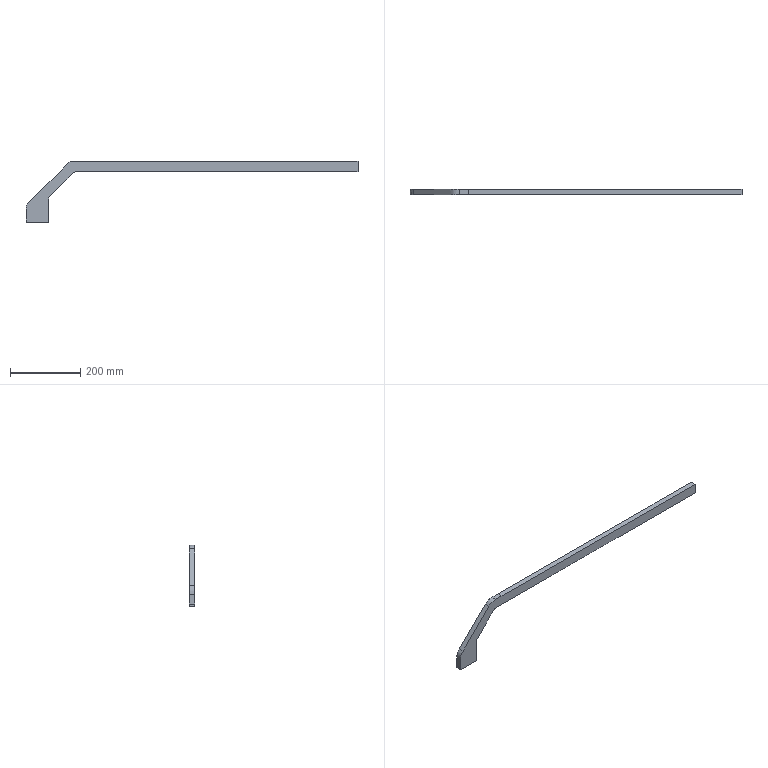Part | NX | features BREP 1 | 1 solid | 18 faces | box 947.785 x 15 x 175.635 mm | volume 489810 mm3 | plane 14 | cylinder 2 | spline 2 | commonest cylinder face diameters 10 x1 20 x1
STEP:
#1=CARTESIAN_POINT('',(752.678,-679.988,1273.821));
#2=VERTEX_POINT('',#1);
#3=CARTESIAN_POINT('',(752.678,-664.988,1273.821));
#4=VERTEX_POINT('',#3);
#5=CARTESIAN_POINT('',(752.678,-672.488,1273.821));
#6=DIRECTION('',(0.,1.,0.));
#7=VECTOR('',#6,1000.);
#8=LINE('',#5,#7);
#9=EDGE_CURVE('',#2,#4,#8,.T.);
#10=ORIENTED_EDGE('',*,*,#9,.T.);
#11=CARTESIAN_POINT('',(754.143,-664.988,1277.356));
#12=VERTEX_POINT('',#11);
#13=CARTESIAN_POINT('',(757.678,-664.988,1273.821));
#14=DIRECTION('',(0.,-1.,0.));
#15=DIRECTION('',(1.,0.,0.));
#16=AXIS2_PLACEMENT_3D('',#13,#14,#15);
#17=CIRCLE('',#16,5.);
#18=EDGE_CURVE('',#12,#4,#17,.T.);
#19=ORIENTED_EDGE('',*,*,#18,.F.);
#20=CARTESIAN_POINT('',(754.143,-679.988,1277.356));
#21=VERTEX_POINT('',#20);
#22=CARTESIAN_POINT('',(754.143,-672.488,1277.356));
#23=DIRECTION('',(0.,1.,0.));
#24=VECTOR('',#23,1000.);
#25=LINE('',#22,#24);
#26=EDGE_CURVE('',#21,#12,#25,.T.);
#27=ORIENTED_EDGE('',*,*,#26,.F.);
#28=CARTESIAN_POINT('',(757.678,-679.988,1273.821));
#29=DIRECTION('',(0.,1.,0.));
#30=DIRECTION('',(1.,0.,0.));
#31=AXIS2_PLACEMENT_3D('',#28,#29,#30);
#32=CIRCLE('',#31,5.);
#33=EDGE_CURVE('',#2,#21,#32,.T.);
#34=ORIENTED_EDGE('',*,*,#33,.F.);
#35=EDGE_LOOP('',(#10,#19,#27,#34));
#36=FACE_BOUND('',#35,.T.);
#37=CARTESIAN_POINT('',(757.678,-672.488,1273.821));
#38=DIRECTION('',(0.,1.,0.));
#39=DIRECTION('',(-1.,0.,0.));
#40=AXIS2_PLACEMENT_3D('',#37,#38,#39);
#41=CYLINDRICAL_SURFACE('',#40,5.);
#42=ADVANCED_FACE('',(#36),#41,.F.);
#43=CARTESIAN_POINT('',(1635.458,-679.988,1378.69));
#44=VERTEX_POINT('',#43);
#45=CARTESIAN_POINT('',(1635.458,-664.988,1378.69));
#46=VERTEX_POINT('',#45);
#47=CARTESIAN_POINT('',(1635.458,-672.488,1378.69));
#48=DIRECTION('',(0.,1.,0.));
#49=VECTOR('',#48,1000.);
#50=LINE('',#47,#49);
#51=EDGE_CURVE('',#44,#46,#50,.T.);
#52=ORIENTED_EDGE('',*,*,#51,.T.);
#53=CARTESIAN_POINT('',(855.477,-664.988,1378.69));
#54=VERTEX_POINT('',#53);
#55=CARTESIAN_POINT('',(1245.467,-664.988,1378.69));
#56=DIRECTION('',(1.,0.,0.));
#57=VECTOR('',#56,1000.);
#58=LINE('',#55,#57);
#59=EDGE_CURVE('',#54,#46,#58,.T.);
#60=ORIENTED_EDGE('',*,*,#59,.F.);
#61=CARTESIAN_POINT('',(855.477,-679.988,1378.69));
#62=VERTEX_POINT('',#61);
#63=CARTESIAN_POINT('',(855.477,-672.488,1378.69));
#64=DIRECTION('',(0.,1.,0.));
#65=VECTOR('',#64,1000.);
#66=LINE('',#63,#65);
#67=EDGE_CURVE('',#62,#54,#66,.T.);
#68=ORIENTED_EDGE('',*,*,#67,.F.);
#69=CARTESIAN_POINT('',(1245.467,-679.988,1378.69));
#70=DIRECTION('',(1.,0.,0.));
#71=VECTOR('',#70,1000.);
#72=LINE('',#69,#71);
#73=EDGE_CURVE('',#62,#44,#72,.T.);
#74=ORIENTED_EDGE('',*,*,#73,.T.);
#75=EDGE_LOOP('',(#52,#60,#68,#74));
#76=FACE_BOUND('',#75,.T.);
#77=CARTESIAN_POINT('',(1245.467,-679.988,1378.69));
#78=DIRECTION('',(0.,0.,1.));
#79=DIRECTION('',(1.,0.,0.));
#80=AXIS2_PLACEMENT_3D('',#77,#78,#79);
#81=PLANE('',#80);
#82=ADVANCED_FACE('',(#76),#81,.T.);
#83=ORIENTED_EDGE('',*,*,#67,.T.);
#84=CARTESIAN_POINT('',(855.475,-664.988,1378.689));
#85=VERTEX_POINT('',#84);
#86=CARTESIAN_POINT('',(855.476,-664.988,1378.689));
#87=DIRECTION('',(0.7071,0.,0.7071));
#88=VECTOR('',#87,1000.);
#89=LINE('',#86,#88);
#90=EDGE_CURVE('',#85,#54,#89,.T.);
#91=ORIENTED_EDGE('',*,*,#90,.F.);
#92=CARTESIAN_POINT('',(855.475,-679.988,1378.689));
#93=VERTEX_POINT('',#92);
#94=CARTESIAN_POINT('',(855.475,-672.488,1378.689));
#95=DIRECTION('',(0.,1.,0.));
#96=VECTOR('',#95,1000.);
#97=LINE('',#94,#96);
#98=EDGE_CURVE('',#93,#85,#97,.T.);
#99=ORIENTED_EDGE('',*,*,#98,.F.);
#100=CARTESIAN_POINT('',(855.476,-679.988,1378.689));
#101=DIRECTION('',(0.7071,0.,0.7071));
#102=VECTOR('',#101,1000.);
#103=LINE('',#100,#102);
#104=EDGE_CURVE('',#93,#62,#103,.T.);
#105=ORIENTED_EDGE('',*,*,#104,.T.);
#106=EDGE_LOOP('',(#83,#91,#99,#105));
#107=FACE_BOUND('',#106,.T.);
#108=CARTESIAN_POINT('',(855.476,-679.988,1378.689));
#109=DIRECTION('',(-0.7071,0.,0.7071));
#110=DIRECTION('',(0.7071,0.,0.7071));
#111=AXIS2_PLACEMENT_3D('',#108,#109,#110);
#112=PLANE('',#111);
#113=ADVANCED_FACE('',(#107),#112,.T.);
#114=ORIENTED_EDGE('',*,*,#98,.T.);
#115=CARTESIAN_POINT('',(829.282,-664.988,1378.689));
#116=VERTEX_POINT('',#115);
#117=CARTESIAN_POINT('',(842.379,-664.988,1378.689));
#118=DIRECTION('',(1.,0.,0.));
#119=VECTOR('',#118,1000.);
#120=LINE('',#117,#119);
#121=EDGE_CURVE('',#116,#85,#120,.T.);
#122=ORIENTED_EDGE('',*,*,#121,.F.);
#123=CARTESIAN_POINT('',(829.282,-679.988,1378.689));
#124=VERTEX_POINT('',#123);
#125=CARTESIAN_POINT('',(829.282,-679.988,1378.689));
#126=DIRECTION('',(0.,1.,0.));
#127=VECTOR('',#126,1000.);
#128=LINE('',#125,#127);
#129=EDGE_CURVE('',#124,#116,#128,.T.);
#130=ORIENTED_EDGE('',*,*,#129,.F.);
#131=CARTESIAN_POINT('',(842.379,-679.988,1378.689));
#132=DIRECTION('',(1.,0.,0.));
#133=VECTOR('',#132,1000.);
#134=LINE('',#131,#133);
#135=EDGE_CURVE('',#124,#93,#134,.T.);
#136=ORIENTED_EDGE('',*,*,#135,.T.);
#137=EDGE_LOOP('',(#114,#122,#130,#136));
#138=FACE_BOUND('',#137,.T.);
#139=CARTESIAN_POINT('',(842.379,-679.988,1378.689));
#140=DIRECTION('',(0.,0.,1.));
#141=DIRECTION('',(1.,0.,0.));
#142=AXIS2_PLACEMENT_3D('',#139,#140,#141);
#143=PLANE('',#142);
#144=ADVANCED_FACE('',(#138),#143,.T.);
#145=ORIENTED_EDGE('',*,*,#129,.T.);
#146=CARTESIAN_POINT('',(802.462,-664.988,1368.101));
#147=VERTEX_POINT('',#146);
#148=CARTESIAN_POINT('',(802.462,-664.988,1368.101));
#149=CARTESIAN_POINT('',(802.713,-664.988,1368.351));
#150=CARTESIAN_POINT('',(803.201,-664.988,1368.831));
#151=CARTESIAN_POINT('',(803.766,-664.988,1369.381));
#152=CARTESIAN_POINT('',(804.526,-664.988,1370.101));
#153=CARTESIAN_POINT('',(805.14,-664.988,1370.666));
#154=CARTESIAN_POINT('',(805.915,-664.988,1371.354));
#155=CARTESIAN_POINT('',(806.881,-664.988,1372.17));
#156=CARTESIAN_POINT('',(808.007,-664.988,1373.064));
#157=CARTESIAN_POINT('',(809.626,-664.988,1374.201));
#158=CARTESIAN_POINT('',(811.67,-664.988,1375.447));
#159=CARTESIAN_POINT('',(813.989,-664.988,1376.546));
#160=CARTESIAN_POINT('',(816.289,-664.988,1377.335));
#161=CARTESIAN_POINT('',(818.163,-664.988,1377.83));
#162=CARTESIAN_POINT('',(819.887,-664.988,1378.167));
#163=CARTESIAN_POINT('',(821.549,-664.988,1378.39));
#164=CARTESIAN_POINT('',(822.722,-664.988,1378.501));
#165=CARTESIAN_POINT('',(823.715,-664.988,1378.574));
#166=CARTESIAN_POINT('',(824.569,-664.988,1378.619));
#167=CARTESIAN_POINT('',(825.586,-664.988,1378.656));
#168=CARTESIAN_POINT('',(826.27,-664.988,1378.67));
#169=CARTESIAN_POINT('',(826.895,-664.988,1378.679));
#170=CARTESIAN_POINT('',(827.459,-664.988,1378.684));
#171=CARTESIAN_POINT('',(827.759,-664.988,1378.686));
#172=CARTESIAN_POINT('',(828.361,-664.988,1378.688));
#173=CARTESIAN_POINT('',(828.884,-664.988,1378.689));
#174=CARTESIAN_POINT('',(829.282,-664.988,1378.689));
#175=B_SPLINE_CURVE_WITH_KNOTS('',3,(#148,#149,#150,#151,#152,#153,#154,#155,#156,#157,#158,#159,#160,#161,#162,#163,#164,#165,#166,#167,#168,#169,#170,#171,#172,#173,#174),.UNSPECIFIED.,.F.,.F.,(4,1,1,1,1,1,1,1,1,1,1,1,1,1,1,1,1,1,1,1,1,1,1,1,4),(0.,0.03125,0.0625,0.09375,0.125,0.1562,0.1875,0.25,0.3125,0.375,0.5,0.5625,0.625,0.6875,0.75,0.7812,0.8125,0.8438,0.875,0.9062,0.9219,0.9375,0.9531,0.9688,1.),.UNSPECIFIED.);
#176=EDGE_CURVE('',#147,#116,#175,.T.);
#177=ORIENTED_EDGE('',*,*,#176,.F.);
#178=CARTESIAN_POINT('',(802.462,-679.988,1368.101));
#179=VERTEX_POINT('',#178);
#180=CARTESIAN_POINT('',(802.462,-672.488,1368.101));
#181=DIRECTION('',(-0.000000001,1.,-0.000000001));
#182=VECTOR('',#181,1000.);
#183=LINE('',#180,#182);
#184=EDGE_CURVE('',#179,#147,#183,.T.);
#185=ORIENTED_EDGE('',*,*,#184,.F.);
#186=CARTESIAN_POINT('',(829.282,-679.988,1378.689));
#187=CARTESIAN_POINT('',(828.885,-679.988,1378.689));
#188=CARTESIAN_POINT('',(828.361,-679.988,1378.688));
#189=CARTESIAN_POINT('',(827.759,-679.988,1378.686));
#190=CARTESIAN_POINT('',(827.458,-679.988,1378.684));
#191=CARTESIAN_POINT('',(826.895,-679.988,1378.679));
#192=CARTESIAN_POINT('',(826.27,-679.988,1378.67));
#193=CARTESIAN_POINT('',(825.586,-679.988,1378.656));
#194=CARTESIAN_POINT('',(824.57,-679.988,1378.619));
#195=CARTESIAN_POINT('',(823.715,-679.988,1378.574));
#196=CARTESIAN_POINT('',(822.723,-679.988,1378.501));
#197=CARTESIAN_POINT('',(821.548,-679.988,1378.39));
#198=CARTESIAN_POINT('',(819.888,-679.988,1378.167));
#199=CARTESIAN_POINT('',(818.163,-679.988,1377.83));
#200=CARTESIAN_POINT('',(816.29,-679.988,1377.335));
#201=CARTESIAN_POINT('',(813.988,-679.988,1376.546));
#202=CARTESIAN_POINT('',(811.67,-679.988,1375.447));
#203=CARTESIAN_POINT('',(809.627,-679.988,1374.202));
#204=CARTESIAN_POINT('',(808.007,-679.988,1373.064));
#205=CARTESIAN_POINT('',(806.882,-679.988,1372.171));
#206=CARTESIAN_POINT('',(805.916,-679.988,1371.355));
#207=CARTESIAN_POINT('',(805.14,-679.988,1370.666));
#208=CARTESIAN_POINT('',(804.527,-679.988,1370.102));
#209=CARTESIAN_POINT('',(803.766,-679.988,1369.381));
#210=CARTESIAN_POINT('',(803.201,-679.988,1368.832));
#211=CARTESIAN_POINT('',(802.713,-679.988,1368.351));
#212=CARTESIAN_POINT('',(802.462,-679.988,1368.101));
#213=B_SPLINE_CURVE_WITH_KNOTS('',3,(#186,#187,#188,#189,#190,#191,#192,#193,#194,#195,#196,#197,#198,#199,#200,#201,#202,#203,#204,#205,#206,#207,#208,#209,#210,#211,#212),.UNSPECIFIED.,.F.,.F.,(4,1,1,1,1,1,1,1,1,1,1,1,1,1,1,1,1,1,1,1,1,1,1,1,4),(0.,0.03125,0.04688,0.0625,0.07812,0.09375,0.125,0.1562,0.1875,0.2188,0.25,0.3125,0.375,0.4375,0.5,0.625,0.6875,0.75,0.8125,0.8438,0.875,0.9062,0.9375,0.9688,1.),.UNSPECIFIED.);
#214=EDGE_CURVE('',#179,#124,#213,.F.);
#215=ORIENTED_EDGE('',*,*,#214,.T.);
#216=EDGE_LOOP('',(#145,#177,#185,#215));
#217=FACE_BOUND('',#216,.T.);
#218=CARTESIAN_POINT('',(802.462,-680.078,1368.101));
#219=CARTESIAN_POINT('',(802.462,-664.988,1368.101));
#220=CARTESIAN_POINT('',(804.233,-680.078,1369.859));
#221=CARTESIAN_POINT('',(804.233,-664.988,1369.859));
#222=CARTESIAN_POINT('',(807.883,-680.078,1373.32));
#223=CARTESIAN_POINT('',(807.883,-664.988,1373.32));
#224=CARTESIAN_POINT('',(814.437,-680.078,1377.09));
#225=CARTESIAN_POINT('',(814.437,-664.988,1377.09));
#226=CARTESIAN_POINT('',(821.879,-680.078,1378.678));
#227=CARTESIAN_POINT('',(821.879,-664.988,1378.678));
#228=CARTESIAN_POINT('',(826.788,-680.078,1378.689));
#229=CARTESIAN_POINT('',(826.788,-664.988,1378.689));
#230=CARTESIAN_POINT('',(829.282,-680.078,1378.689));
#231=CARTESIAN_POINT('',(829.282,-664.988,1378.689));
#232=B_SPLINE_SURFACE_WITH_KNOTS('',3,1,((#218,#219),(#220,#221),(#222,#223),(#224,#225),(#226,#227),(#228,#229),(#230,#231)),.SURF_OF_LINEAR_EXTRUSION.,.F.,.F.,.F.,(4,1,1,1,4),(2,2),(0.009839,7.507,15.005,22.502,30.),(0.,1.),.UNSPECIFIED.);
#233=ADVANCED_FACE('',(#217),#232,.T.);
#234=ORIENTED_EDGE('',*,*,#184,.T.);
#235=CARTESIAN_POINT('',(698.27,-664.988,1263.91));
#236=VERTEX_POINT('',#235);
#237=CARTESIAN_POINT('',(750.366,-664.988,1316.006));
#238=DIRECTION('',(0.7071,0.,0.7071));
#239=VECTOR('',#238,1000.);
#240=LINE('',#237,#239);
#241=EDGE_CURVE('',#236,#147,#240,.T.);
#242=ORIENTED_EDGE('',*,*,#241,.F.);
#243=CARTESIAN_POINT('',(698.27,-679.988,1263.91));
#244=VERTEX_POINT('',#243);
#245=CARTESIAN_POINT('',(698.27,-679.988,1263.91));
#246=DIRECTION('',(0.,1.,0.));
#247=VECTOR('',#246,1000.);
#248=LINE('',#245,#247);
#249=EDGE_CURVE('',#244,#236,#248,.T.);
#250=ORIENTED_EDGE('',*,*,#249,.F.);
#251=CARTESIAN_POINT('',(750.366,-679.988,1316.006));
#252=DIRECTION('',(0.7071,0.,0.7071));
#253=VECTOR('',#252,1000.);
#254=LINE('',#251,#253);
#255=EDGE_CURVE('',#244,#179,#254,.T.);
#256=ORIENTED_EDGE('',*,*,#255,.T.);
#257=EDGE_LOOP('',(#234,#242,#250,#256));
#258=FACE_BOUND('',#257,.T.);
#259=CARTESIAN_POINT('',(750.366,-679.988,1316.006));
#260=DIRECTION('',(0.7071,0.,-0.7071));
#261=DIRECTION('',(0.7071,0.,0.7071));
#262=AXIS2_PLACEMENT_3D('',#259,#260,#261);
#263=PLANE('',#262);
#264=ADVANCED_FACE('',(#258),#263,.F.);
#265=ORIENTED_EDGE('',*,*,#249,.T.);
#266=CARTESIAN_POINT('',(687.713,-664.988,1240.892));
#267=VERTEX_POINT('',#266);
#268=CARTESIAN_POINT('',(687.713,-664.988,1240.892));
#269=CARTESIAN_POINT('',(687.73,-664.988,1241.481));
#270=CARTESIAN_POINT('',(687.784,-664.988,1242.634));
#271=CARTESIAN_POINT('',(687.896,-664.988,1244.111));
#272=CARTESIAN_POINT('',(688.103,-664.988,1245.85));
#273=CARTESIAN_POINT('',(688.36,-664.988,1247.36));
#274=CARTESIAN_POINT('',(688.735,-664.988,1249.013));
#275=CARTESIAN_POINT('',(689.327,-664.988,1251.048));
#276=CARTESIAN_POINT('',(690.152,-664.988,1253.12));
#277=CARTESIAN_POINT('',(691.126,-664.988,1255.013));
#278=CARTESIAN_POINT('',(691.989,-664.988,1256.459));
#279=CARTESIAN_POINT('',(692.852,-664.988,1257.738));
#280=CARTESIAN_POINT('',(693.907,-664.988,1259.135));
#281=CARTESIAN_POINT('',(694.838,-664.988,1260.259));
#282=CARTESIAN_POINT('',(695.851,-664.988,1261.396));
#283=CARTESIAN_POINT('',(696.523,-664.988,1262.114));
#284=CARTESIAN_POINT('',(697.15,-664.988,1262.77));
#285=CARTESIAN_POINT('',(697.637,-664.988,1263.269));
#286=CARTESIAN_POINT('',(698.054,-664.988,1263.692));
#287=CARTESIAN_POINT('',(698.27,-664.988,1263.91));
#288=B_SPLINE_CURVE_WITH_KNOTS('',3,(#268,#269,#270,#271,#272,#273,#274,#275,#276,#277,#278,#279,#280,#281,#282,#283,#284,#285,#286,#287),.UNSPECIFIED.,.F.,.F.,(4,1,1,1,1,1,1,1,1,1,1,1,1,1,1,1,1,4),(0.,0.0625,0.125,0.1875,0.25,0.3125,0.375,0.5,0.5625,0.625,0.6875,0.75,0.8125,0.875,0.9062,0.9375,0.9688,1.),.UNSPECIFIED.);
#289=EDGE_CURVE('',#267,#236,#288,.T.);
#290=ORIENTED_EDGE('',*,*,#289,.F.);
#291=CARTESIAN_POINT('',(687.674,-664.988,1237.08));
#292=VERTEX_POINT('',#291);
#293=CARTESIAN_POINT('',(687.674,-664.988,1237.08));
#294=CARTESIAN_POINT('',(687.674,-664.988,1237.501));
#295=CARTESIAN_POINT('',(687.674,-664.988,1238.045));
#296=CARTESIAN_POINT('',(687.677,-664.988,1238.654));
#297=CARTESIAN_POINT('',(687.678,-664.988,1238.934));
#298=CARTESIAN_POINT('',(687.684,-664.988,1239.516));
#299=CARTESIAN_POINT('',(687.693,-664.988,1240.145));
#300=CARTESIAN_POINT('',(687.704,-664.988,1240.607));
#301=CARTESIAN_POINT('',(687.713,-664.988,1240.892));
#302=B_SPLINE_CURVE_WITH_KNOTS('',3,(#293,#294,#295,#296,#297,#298,#299,#300,#301),.UNSPECIFIED.,.F.,.F.,(4,1,1,1,1,1,4),(0.,0.25,0.375,0.5,0.625,0.75,1.),.UNSPECIFIED.);
#303=EDGE_CURVE('',#292,#267,#302,.T.);
#304=ORIENTED_EDGE('',*,*,#303,.F.);
#305=CARTESIAN_POINT('',(687.674,-679.988,1237.08));
#306=VERTEX_POINT('',#305);
#307=CARTESIAN_POINT('',(687.674,-672.488,1237.08));
#308=DIRECTION('',(0.,1.,0.));
#309=VECTOR('',#308,1000.);
#310=LINE('',#307,#309);
#311=EDGE_CURVE('',#306,#292,#310,.T.);
#312=ORIENTED_EDGE('',*,*,#311,.F.);
#313=CARTESIAN_POINT('',(687.713,-679.988,1240.892));
#314=VERTEX_POINT('',#313);
#315=CARTESIAN_POINT('',(687.713,-679.988,1240.892));
#316=CARTESIAN_POINT('',(687.704,-679.988,1240.607));
#317=CARTESIAN_POINT('',(687.693,-679.988,1240.146));
#318=CARTESIAN_POINT('',(687.684,-679.988,1239.516));
#319=CARTESIAN_POINT('',(687.678,-679.988,1238.933));
#320=CARTESIAN_POINT('',(687.677,-679.988,1238.655));
#321=CARTESIAN_POINT('',(687.674,-679.988,1238.045));
#322=CARTESIAN_POINT('',(687.674,-679.988,1237.501));
#323=CARTESIAN_POINT('',(687.674,-679.988,1237.08));
#324=B_SPLINE_CURVE_WITH_KNOTS('',3,(#315,#316,#317,#318,#319,#320,#321,#322,#323),.UNSPECIFIED.,.F.,.F.,(4,1,1,1,1,1,4),(0.,0.25,0.375,0.5,0.625,0.75,1.),.UNSPECIFIED.);
#325=EDGE_CURVE('',#306,#314,#324,.F.);
#326=ORIENTED_EDGE('',*,*,#325,.T.);
#327=CARTESIAN_POINT('',(698.27,-679.988,1263.91));
#328=CARTESIAN_POINT('',(698.054,-679.988,1263.692));
#329=CARTESIAN_POINT('',(697.637,-679.988,1263.27));
#330=CARTESIAN_POINT('',(697.149,-679.988,1262.77));
#331=CARTESIAN_POINT('',(696.524,-679.988,1262.115));
#332=CARTESIAN_POINT('',(695.851,-679.988,1261.395));
#333=CARTESIAN_POINT('',(694.839,-679.988,1260.26));
#334=CARTESIAN_POINT('',(693.907,-679.988,1259.134));
#335=CARTESIAN_POINT('',(692.853,-679.988,1257.739));
#336=CARTESIAN_POINT('',(691.989,-679.988,1256.459));
#337=CARTESIAN_POINT('',(691.126,-679.988,1255.013));
#338=CARTESIAN_POINT('',(690.152,-679.988,1253.12));
#339=CARTESIAN_POINT('',(689.327,-679.988,1251.048));
#340=CARTESIAN_POINT('',(688.735,-679.988,1249.014));
#341=CARTESIAN_POINT('',(688.36,-679.988,1247.359));
#342=CARTESIAN_POINT('',(688.104,-679.988,1245.851));
#343=CARTESIAN_POINT('',(687.896,-679.988,1244.111));
#344=CARTESIAN_POINT('',(687.784,-679.988,1242.634));
#345=CARTESIAN_POINT('',(687.73,-679.988,1241.481));
#346=CARTESIAN_POINT('',(687.713,-679.988,1240.892));
#347=B_SPLINE_CURVE_WITH_KNOTS('',3,(#327,#328,#329,#330,#331,#332,#333,#334,#335,#336,#337,#338,#339,#340,#341,#342,#343,#344,#345,#346),.UNSPECIFIED.,.F.,.F.,(4,1,1,1,1,1,1,1,1,1,1,1,1,1,1,1,1,4),(0.,0.03125,0.0625,0.09375,0.125,0.1875,0.25,0.3125,0.375,0.4375,0.5,0.625,0.6875,0.75,0.8125,0.875,0.9375,1.),.UNSPECIFIED.);
#348=EDGE_CURVE('',#314,#244,#347,.F.);
#349=ORIENTED_EDGE('',*,*,#348,.T.);
#350=EDGE_LOOP('',(#265,#290,#304,#312,#326,#349));
#351=FACE_BOUND('',#350,.T.);
#352=CARTESIAN_POINT('',(687.674,-679.988,1237.08));
#353=CARTESIAN_POINT('',(687.674,-664.988,1237.08));
#354=CARTESIAN_POINT('',(687.674,-679.988,1239.588));
#355=CARTESIAN_POINT('',(687.674,-664.988,1239.588));
#356=CARTESIAN_POINT('',(687.693,-679.988,1244.589));
#357=CARTESIAN_POINT('',(687.693,-664.988,1244.589));
#358=CARTESIAN_POINT('',(689.287,-679.988,1251.958));
#359=CARTESIAN_POINT('',(689.287,-664.988,1251.958));
#360=CARTESIAN_POINT('',(693.086,-679.988,1258.533));
#361=CARTESIAN_POINT('',(693.086,-664.988,1258.533));
#362=CARTESIAN_POINT('',(696.506,-679.988,1262.133));
#363=CARTESIAN_POINT('',(696.506,-664.988,1262.133));
#364=CARTESIAN_POINT('',(698.27,-679.988,1263.91));
#365=CARTESIAN_POINT('',(698.27,-664.988,1263.91));
#366=B_SPLINE_SURFACE_WITH_KNOTS('',3,1,((#352,#353),(#354,#355),(#356,#357),(#358,#359),(#360,#361),(#362,#363),(#364,#365)),.SURF_OF_LINEAR_EXTRUSION.,.F.,.F.,.F.,(4,1,1,1,4),(2,2),(0.,7.493,14.985,22.478,29.971),(0.,1.),.UNSPECIFIED.);
#367=ADVANCED_FACE('',(#351),#366,.T.);
#368=ORIENTED_EDGE('',*,*,#311,.T.);
#369=CARTESIAN_POINT('',(687.674,-664.988,1210.887));
#370=VERTEX_POINT('',#369);
#371=CARTESIAN_POINT('',(687.674,-664.988,1223.984));
#372=DIRECTION('',(0.,0.,1.));
#373=VECTOR('',#372,1000.);
#374=LINE('',#371,#373);
#375=EDGE_CURVE('',#370,#292,#374,.T.);
#376=ORIENTED_EDGE('',*,*,#375,.F.);
#377=CARTESIAN_POINT('',(687.674,-679.988,1210.887));
#378=VERTEX_POINT('',#377);
#379=CARTESIAN_POINT('',(687.674,-672.488,1210.887));
#380=DIRECTION('',(0.,-1.,0.));
#381=VECTOR('',#380,1000.);
#382=LINE('',#379,#381);
#383=EDGE_CURVE('',#370,#378,#382,.T.);
#384=ORIENTED_EDGE('',*,*,#383,.T.);
#385=CARTESIAN_POINT('',(687.674,-679.988,1223.984));
#386=DIRECTION('',(0.,0.,1.));
#387=VECTOR('',#386,1000.);
#388=LINE('',#385,#387);
#389=EDGE_CURVE('',#378,#306,#388,.T.);
#390=ORIENTED_EDGE('',*,*,#389,.T.);
#391=EDGE_LOOP('',(#368,#376,#384,#390));
#392=FACE_BOUND('',#391,.T.);
#393=CARTESIAN_POINT('',(687.674,-679.988,1223.984));
#394=DIRECTION('',(1.,0.,0.));
#395=DIRECTION('',(0.,1.,0.));
#396=AXIS2_PLACEMENT_3D('',#393,#394,#395);
#397=PLANE('',#396);
#398=ADVANCED_FACE('',(#392),#397,.F.);
#399=CARTESIAN_POINT('',(687.678,-679.988,1210.892));
#400=VERTEX_POINT('',#399);
#401=CARTESIAN_POINT('',(687.676,-679.988,1210.889));
#402=DIRECTION('',(0.7071,0.,0.7071));
#403=VECTOR('',#402,1000.);
#404=LINE('',#401,#403);
#405=EDGE_CURVE('',#378,#400,#404,.T.);
#406=ORIENTED_EDGE('',*,*,#405,.F.);
#407=ORIENTED_EDGE('',*,*,#383,.F.);
#408=CARTESIAN_POINT('',(687.678,-664.988,1210.892));
#409=VERTEX_POINT('',#408);
#410=CARTESIAN_POINT('',(687.676,-664.988,1210.889));
#411=DIRECTION('',(0.7071,0.,0.7071));
#412=VECTOR('',#411,1000.);
#413=LINE('',#410,#412);
#414=EDGE_CURVE('',#370,#409,#413,.T.);
#415=ORIENTED_EDGE('',*,*,#414,.T.);
#416=CARTESIAN_POINT('',(687.678,-672.488,1210.892));
#417=DIRECTION('',(0.,-1.,0.));
#418=VECTOR('',#417,1000.);
#419=LINE('',#416,#418);
#420=EDGE_CURVE('',#409,#400,#419,.T.);
#421=ORIENTED_EDGE('',*,*,#420,.T.);
#422=EDGE_LOOP('',(#406,#407,#415,#421));
#423=FACE_BOUND('',#422,.T.);
#424=CARTESIAN_POINT('',(687.676,-679.988,1210.889));
#425=DIRECTION('',(0.7071,0.,-0.7071));
#426=DIRECTION('',(0.7071,0.,0.7071));
#427=AXIS2_PLACEMENT_3D('',#424,#425,#426);
#428=PLANE('',#427);
#429=ADVANCED_FACE('',(#423),#428,.T.);
#430=CARTESIAN_POINT('',(687.678,-679.988,1203.055));
#431=VERTEX_POINT('',#430);
#432=CARTESIAN_POINT('',(687.678,-679.988,1206.973));
#433=DIRECTION('',(0.,0.,1.));
#434=VECTOR('',#433,1000.);
#435=LINE('',#432,#434);
#436=EDGE_CURVE('',#431,#400,#435,.T.);
#437=ORIENTED_EDGE('',*,*,#436,.T.);
#438=ORIENTED_EDGE('',*,*,#420,.F.);
#439=CARTESIAN_POINT('',(687.678,-664.988,1203.055));
#440=VERTEX_POINT('',#439);
#441=CARTESIAN_POINT('',(687.678,-664.988,1206.973));
#442=DIRECTION('',(0.,0.,1.));
#443=VECTOR('',#442,1000.);
#444=LINE('',#441,#443);
#445=EDGE_CURVE('',#440,#409,#444,.T.);
#446=ORIENTED_EDGE('',*,*,#445,.F.);
#447=CARTESIAN_POINT('',(687.678,-672.488,1203.055));
#448=DIRECTION('',(0.,1.,0.));
#449=VECTOR('',#448,1000.);
#450=LINE('',#447,#449);
#451=EDGE_CURVE('',#431,#440,#450,.T.);
#452=ORIENTED_EDGE('',*,*,#451,.F.);
#453=EDGE_LOOP('',(#437,#438,#446,#452));
#454=FACE_BOUND('',#453,.T.);
#455=CARTESIAN_POINT('',(687.678,-679.988,655.446));
#456=DIRECTION('',(-1.,0.,0.));
#457=DIRECTION('',(0.,1.,0.));
#458=AXIS2_PLACEMENT_3D('',#455,#456,#457);
#459=PLANE('',#458);
#460=ADVANCED_FACE('',(#454),#459,.T.);
#461=ORIENTED_EDGE('',*,*,#451,.T.);
#462=CARTESIAN_POINT('',(752.678,-664.988,1203.055));
#463=VERTEX_POINT('',#462);
#464=CARTESIAN_POINT('',(720.178,-664.988,1203.055));
#465=DIRECTION('',(1.,0.,0.));
#466=VECTOR('',#465,1000.);
#467=LINE('',#464,#466);
#468=EDGE_CURVE('',#440,#463,#467,.T.);
#469=ORIENTED_EDGE('',*,*,#468,.T.);
#470=CARTESIAN_POINT('',(752.678,-679.988,1203.055));
#471=VERTEX_POINT('',#470);
#472=CARTESIAN_POINT('',(752.678,-672.488,1203.055));
#473=DIRECTION('',(0.,1.,0.));
#474=VECTOR('',#473,1000.);
#475=LINE('',#472,#474);
#476=EDGE_CURVE('',#471,#463,#475,.T.);
#477=ORIENTED_EDGE('',*,*,#476,.F.);
#478=CARTESIAN_POINT('',(720.178,-679.988,1203.055));
#479=DIRECTION('',(1.,0.,0.));
#480=VECTOR('',#479,1000.);
#481=LINE('',#478,#480);
#482=EDGE_CURVE('',#431,#471,#481,.T.);
#483=ORIENTED_EDGE('',*,*,#482,.F.);
#484=EDGE_LOOP('',(#461,#469,#477,#483));
#485=FACE_BOUND('',#484,.T.);
#486=CARTESIAN_POINT('',(717.678,-679.988,1203.055));
#487=DIRECTION('',(0.,0.,-1.));
#488=DIRECTION('',(1.,0.,0.));
#489=AXIS2_PLACEMENT_3D('',#486,#487,#488);
#490=PLANE('',#489);
#491=ADVANCED_FACE('',(#485),#490,.T.);
#492=ORIENTED_EDGE('',*,*,#9,.F.);
#493=CARTESIAN_POINT('',(752.678,-679.988,1238.438));
#494=DIRECTION('',(0.,0.,-1.));
#495=VECTOR('',#494,1000.);
#496=LINE('',#493,#495);
#497=EDGE_CURVE('',#2,#471,#496,.T.);
#498=ORIENTED_EDGE('',*,*,#497,.T.);
#499=ORIENTED_EDGE('',*,*,#476,.T.);
#500=CARTESIAN_POINT('',(752.678,-664.988,1238.438));
#501=DIRECTION('',(0.,0.,-1.));
#502=VECTOR('',#501,1000.);
#503=LINE('',#500,#502);
#504=EDGE_CURVE('',#4,#463,#503,.T.);
#505=ORIENTED_EDGE('',*,*,#504,.F.);
#506=EDGE_LOOP('',(#492,#498,#499,#505));
#507=FACE_BOUND('',#506,.T.);
#508=CARTESIAN_POINT('',(752.678,-672.488,1203.055));
#509=DIRECTION('',(-1.,0.,0.));
#510=DIRECTION('',(0.,1.,0.));
#511=AXIS2_PLACEMENT_3D('',#508,#509,#510);
#512=PLANE('',#511);
#513=ADVANCED_FACE('',(#507),#512,.F.);
#514=CARTESIAN_POINT('',(822.548,-664.988,1345.761));
#515=VERTEX_POINT('',#514);
#516=CARTESIAN_POINT('',(788.345,-664.988,1311.559));
#517=DIRECTION('',(0.7071,0.,0.7071));
#518=VECTOR('',#517,1000.);
#519=LINE('',#516,#518);
#520=EDGE_CURVE('',#12,#515,#519,.T.);
#521=ORIENTED_EDGE('',*,*,#520,.T.);
#522=CARTESIAN_POINT('',(822.548,-679.988,1345.761));
#523=VERTEX_POINT('',#522);
#524=CARTESIAN_POINT('',(822.548,-672.488,1345.761));
#525=DIRECTION('',(0.,-1.,0.));
#526=VECTOR('',#525,1000.);
#527=LINE('',#524,#526);
#528=EDGE_CURVE('',#515,#523,#527,.T.);
#529=ORIENTED_EDGE('',*,*,#528,.T.);
#530=CARTESIAN_POINT('',(788.345,-679.988,1311.559));
#531=DIRECTION('',(0.7071,0.,0.7071));
#532=VECTOR('',#531,1000.);
#533=LINE('',#530,#532);
#534=EDGE_CURVE('',#21,#523,#533,.T.);
#535=ORIENTED_EDGE('',*,*,#534,.F.);
#536=ORIENTED_EDGE('',*,*,#26,.T.);
#537=EDGE_LOOP('',(#521,#529,#535,#536));
#538=FACE_BOUND('',#537,.T.);
#539=CARTESIAN_POINT('',(771.577,-679.988,1294.791));
#540=DIRECTION('',(0.7071,0.,-0.7071));
#541=DIRECTION('',(0.7071,0.,0.7071));
#542=AXIS2_PLACEMENT_3D('',#539,#540,#541);
#543=PLANE('',#542);
#544=ADVANCED_FACE('',(#538),#543,.T.);
#545=ORIENTED_EDGE('',*,*,#534,.T.);
#546=CARTESIAN_POINT('',(829.619,-679.988,1348.69));
#547=VERTEX_POINT('',#546);
#548=CARTESIAN_POINT('',(829.619,-679.988,1338.69));
#549=DIRECTION('',(0.,-1.,0.));
#550=DIRECTION('',(1.,0.,0.));
#551=AXIS2_PLACEMENT_3D('',#548,#549,#550);
#552=CIRCLE('',#551,10.);
#553=EDGE_CURVE('',#547,#523,#552,.T.);
#554=ORIENTED_EDGE('',*,*,#553,.F.);
#555=CARTESIAN_POINT('',(1635.458,-679.988,1348.69));
#556=VERTEX_POINT('',#555);
#557=CARTESIAN_POINT('',(1232.539,-679.988,1348.69));
#558=DIRECTION('',(1.,0.,0.));
#559=VECTOR('',#558,1000.);
#560=LINE('',#557,#559);
#561=EDGE_CURVE('',#547,#556,#560,.T.);
#562=ORIENTED_EDGE('',*,*,#561,.T.);
#563=CARTESIAN_POINT('',(1635.458,-679.988,1363.69));
#564=DIRECTION('',(0.,0.,-1.));
#565=VECTOR('',#564,1000.);
#566=LINE('',#563,#565);
#567=EDGE_CURVE('',#44,#556,#566,.T.);
#568=ORIENTED_EDGE('',*,*,#567,.F.);
#569=ORIENTED_EDGE('',*,*,#73,.F.);
#570=ORIENTED_EDGE('',*,*,#104,.F.);
#571=ORIENTED_EDGE('',*,*,#135,.F.);
#572=ORIENTED_EDGE('',*,*,#214,.F.);
#573=ORIENTED_EDGE('',*,*,#255,.F.);
#574=ORIENTED_EDGE('',*,*,#348,.F.);
#575=ORIENTED_EDGE('',*,*,#325,.F.);
#576=ORIENTED_EDGE('',*,*,#389,.F.);
#577=ORIENTED_EDGE('',*,*,#405,.T.);
#578=ORIENTED_EDGE('',*,*,#436,.F.);
#579=ORIENTED_EDGE('',*,*,#482,.T.);
#580=ORIENTED_EDGE('',*,*,#497,.F.);
#581=ORIENTED_EDGE('',*,*,#33,.T.);
#582=EDGE_LOOP('',(#545,#554,#562,#568,#569,#570,#571,#572,#573,#574,#575,#576,#577,#578,#579,#580,#581));
#583=FACE_BOUND('',#582,.T.);
#584=CARTESIAN_POINT('',(1125.65,-679.988,1648.863));
#585=DIRECTION('',(0.,1.,0.));
#586=DIRECTION('',(-0.7071,0.,0.7071));
#587=AXIS2_PLACEMENT_3D('',#584,#585,#586);
#588=PLANE('',#587);
#589=ADVANCED_FACE('',(#583),#588,.F.);
#590=CARTESIAN_POINT('',(1635.458,-664.988,1348.69));
#591=VERTEX_POINT('',#590);
#592=CARTESIAN_POINT('',(1635.458,-672.488,1348.69));
#593=DIRECTION('',(0.,1.,0.));
#594=VECTOR('',#593,1000.);
#595=LINE('',#592,#594);
#596=EDGE_CURVE('',#556,#591,#595,.T.);
#597=ORIENTED_EDGE('',*,*,#596,.T.);
#598=CARTESIAN_POINT('',(1635.458,-664.988,1363.69));
#599=DIRECTION('',(0.,0.,-1.));
#600=VECTOR('',#599,1000.);
#601=LINE('',#598,#600);
#602=EDGE_CURVE('',#46,#591,#601,.T.);
#603=ORIENTED_EDGE('',*,*,#602,.F.);
#604=ORIENTED_EDGE('',*,*,#51,.F.);
#605=ORIENTED_EDGE('',*,*,#567,.T.);
#606=EDGE_LOOP('',(#597,#603,#604,#605));
#607=FACE_BOUND('',#606,.T.);
#608=CARTESIAN_POINT('',(1635.458,-679.988,1363.69));
#609=DIRECTION('',(-1.,0.,0.));
#610=DIRECTION('',(0.,1.,0.));
#611=AXIS2_PLACEMENT_3D('',#608,#609,#610);
#612=PLANE('',#611);
#613=ADVANCED_FACE('',(#607),#612,.F.);
#614=ORIENTED_EDGE('',*,*,#504,.T.);
#615=ORIENTED_EDGE('',*,*,#468,.F.);
#616=ORIENTED_EDGE('',*,*,#445,.T.);
#617=ORIENTED_EDGE('',*,*,#414,.F.);
#618=ORIENTED_EDGE('',*,*,#375,.T.);
#619=ORIENTED_EDGE('',*,*,#303,.T.);
#620=ORIENTED_EDGE('',*,*,#289,.T.);
#621=ORIENTED_EDGE('',*,*,#241,.T.);
#622=ORIENTED_EDGE('',*,*,#176,.T.);
#623=ORIENTED_EDGE('',*,*,#121,.T.);
#624=ORIENTED_EDGE('',*,*,#90,.T.);
#625=ORIENTED_EDGE('',*,*,#59,.T.);
#626=ORIENTED_EDGE('',*,*,#602,.T.);
#627=CARTESIAN_POINT('',(829.619,-664.988,1348.69));
#628=VERTEX_POINT('',#627);
#629=CARTESIAN_POINT('',(1232.539,-664.988,1348.69));
#630=DIRECTION('',(1.,0.,0.));
#631=VECTOR('',#630,1000.);
#632=LINE('',#629,#631);
#633=EDGE_CURVE('',#628,#591,#632,.T.);
#634=ORIENTED_EDGE('',*,*,#633,.F.);
#635=CARTESIAN_POINT('',(829.619,-664.988,1338.69));
#636=DIRECTION('',(0.,-1.,0.));
#637=DIRECTION('',(1.,0.,0.));
#638=AXIS2_PLACEMENT_3D('',#635,#636,#637);
#639=CIRCLE('',#638,10.);
#640=EDGE_CURVE('',#628,#515,#639,.T.);
#641=ORIENTED_EDGE('',*,*,#640,.T.);
#642=ORIENTED_EDGE('',*,*,#520,.F.);
#643=ORIENTED_EDGE('',*,*,#18,.T.);
#644=EDGE_LOOP('',(#614,#615,#616,#617,#618,#619,#620,#621,#622,#623,#624,#625,#626,#634,#641,#642,#643));
#645=FACE_BOUND('',#644,.T.);
#646=CARTESIAN_POINT('',(720.178,-664.988,1203.055));
#647=DIRECTION('',(0.,-1.,0.));
#648=DIRECTION('',(1.,0.,0.));
#649=AXIS2_PLACEMENT_3D('',#646,#647,#648);
#650=PLANE('',#649);
#651=ADVANCED_FACE('',(#645),#650,.F.);
#652=CARTESIAN_POINT('',(829.619,-672.488,1348.69));
#653=DIRECTION('',(0.,-1.,0.));
#654=VECTOR('',#653,1000.);
#655=LINE('',#652,#654);
#656=EDGE_CURVE('',#628,#547,#655,.T.);
#657=ORIENTED_EDGE('',*,*,#656,.T.);
#658=ORIENTED_EDGE('',*,*,#553,.T.);
#659=ORIENTED_EDGE('',*,*,#528,.F.);
#660=ORIENTED_EDGE('',*,*,#640,.F.);
#661=EDGE_LOOP('',(#657,#658,#659,#660));
#662=FACE_BOUND('',#661,.T.);
#663=CARTESIAN_POINT('',(829.619,-672.488,1338.69));
#664=DIRECTION('',(0.,-1.,0.));
#665=DIRECTION('',(0.,0.,1.));
#666=AXIS2_PLACEMENT_3D('',#663,#664,#665);
#667=CYLINDRICAL_SURFACE('',#666,10.);
#668=ADVANCED_FACE('',(#662),#667,.F.);
#669=ORIENTED_EDGE('',*,*,#656,.F.);
#670=ORIENTED_EDGE('',*,*,#633,.T.);
#671=ORIENTED_EDGE('',*,*,#596,.F.);
#672=ORIENTED_EDGE('',*,*,#561,.F.);
#673=EDGE_LOOP('',(#669,#670,#671,#672));
#674=FACE_BOUND('',#673,.T.);
#675=CARTESIAN_POINT('',(1230.467,-679.988,1348.69));
#676=DIRECTION('',(0.,0.,1.));
#677=DIRECTION('',(1.,0.,0.));
#678=AXIS2_PLACEMENT_3D('',#675,#676,#677);
#679=PLANE('',#678);
#680=ADVANCED_FACE('',(#674),#679,.F.);
#681=CLOSED_SHELL('',(#42,#82,#113,#144,#233,#264,#367,#398,#429,#460,#491,#513,#544,#589,#613,#651,#668,#680));
#682=MANIFOLD_SOLID_BREP('',#681);
#683=(LENGTH_UNIT()NAMED_UNIT(*)SI_UNIT(.MILLI.,.METRE.));
#684=UNCERTAINTY_MEASURE_WITH_UNIT(LENGTH_MEASURE(0.0508),#683,'','');
#685=(NAMED_UNIT(*)PLANE_ANGLE_UNIT()SI_UNIT($,.RADIAN.));
#686=(NAMED_UNIT(*)SI_UNIT($,.STERADIAN.)SOLID_ANGLE_UNIT());
#687=(GEOMETRIC_REPRESENTATION_CONTEXT(3)GLOBAL_UNCERTAINTY_ASSIGNED_CONTEXT((#684))GLOBAL_UNIT_ASSIGNED_CONTEXT((#683,#685,#686))REPRESENTATION_CONTEXT('',''));
#688=ADVANCED_BREP_SHAPE_REPRESENTATION('',(#682),#687);